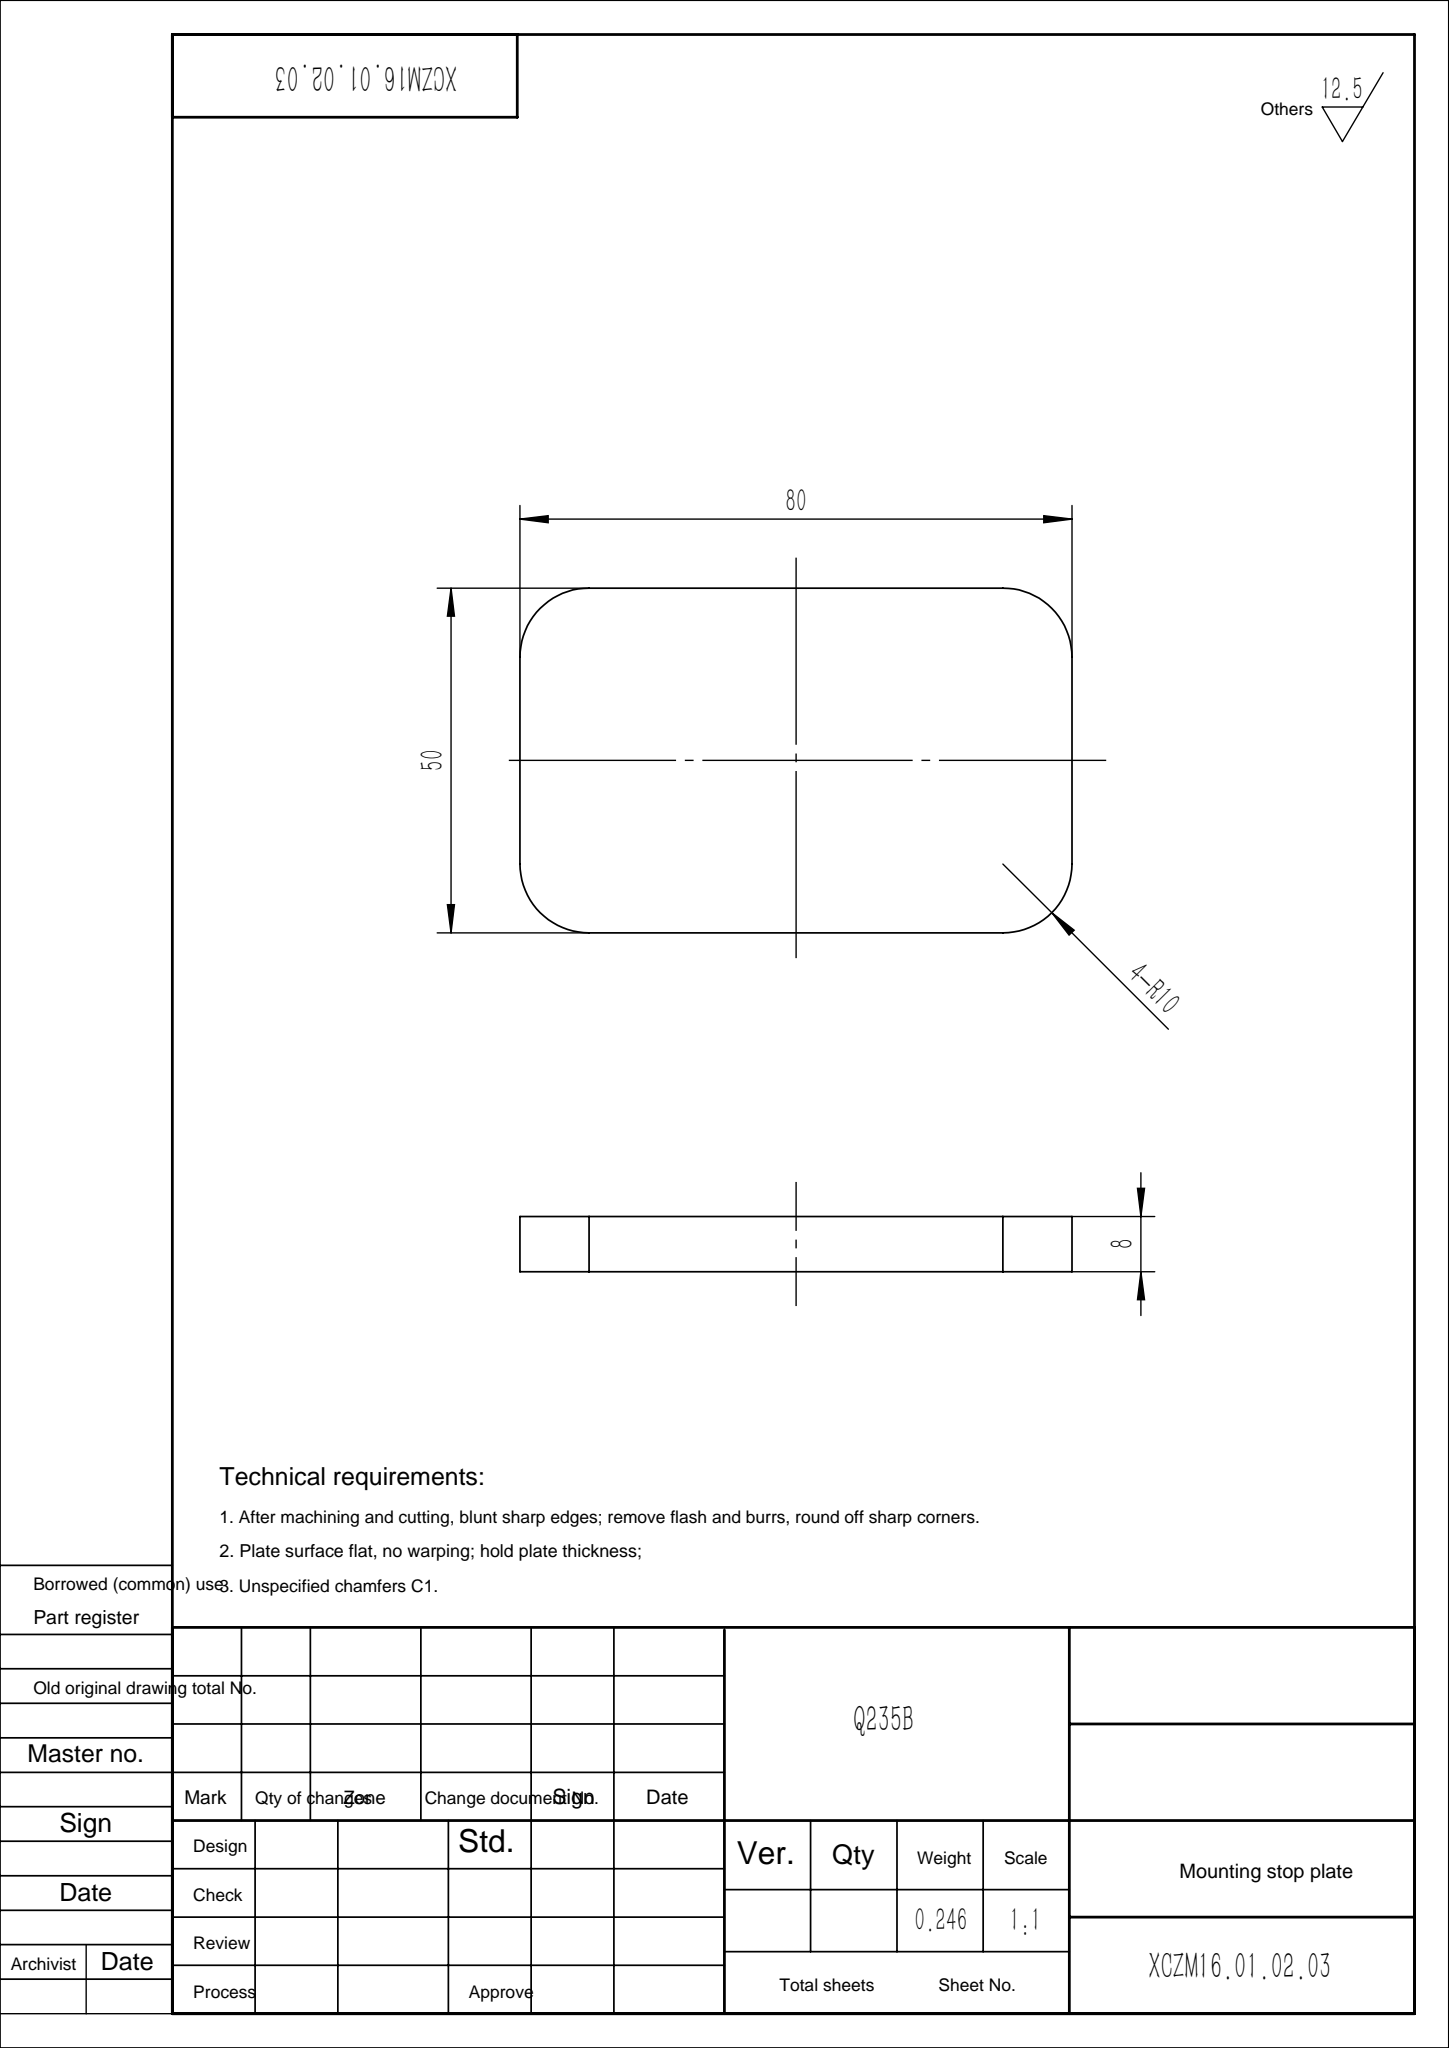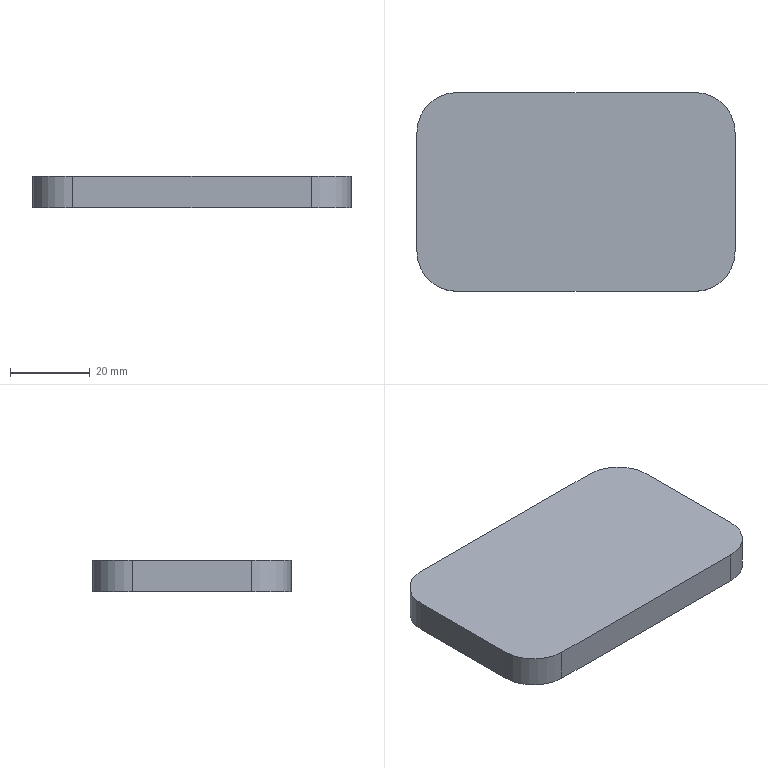Part | SolidWorks | features Extrusion 1 | 1 solid | 10 faces | box 80 x 50 x 8 mm | volume 31313 mm3 | plane 6 | cylinder 4 | commonest cylinder face diameters 20 x4
STEP:
#1=CARTESIAN_POINT('',(-40.,-15.,0.));
#2=VERTEX_POINT('',#1);
#3=CARTESIAN_POINT('',(-30.,-25.,0.));
#4=VERTEX_POINT('',#3);
#5=CARTESIAN_POINT('',(-30.,-15.,0.));
#6=DIRECTION('',(0.,0.,1.));
#7=DIRECTION('',(-1.,0.,0.));
#8=AXIS2_PLACEMENT_3D('',#5,#6,#7);
#9=CIRCLE('',#8,10.);
#10=EDGE_CURVE('',#2,#4,#9,.T.);
#11=ORIENTED_EDGE('',*,*,#10,.T.);
#12=CARTESIAN_POINT('',(-30.,-25.,8.));
#13=VERTEX_POINT('',#12);
#14=CARTESIAN_POINT('',(-30.,-25.,8.));
#15=DIRECTION('',(0.,0.,-1.));
#16=VECTOR('',#15,1000.);
#17=LINE('',#14,#16);
#18=EDGE_CURVE('',#13,#4,#17,.T.);
#19=ORIENTED_EDGE('',*,*,#18,.F.);
#20=CARTESIAN_POINT('',(-40.,-15.,8.));
#21=VERTEX_POINT('',#20);
#22=CARTESIAN_POINT('',(-30.,-15.,8.));
#23=DIRECTION('',(0.,0.,1.));
#24=DIRECTION('',(-1.,0.,0.));
#25=AXIS2_PLACEMENT_3D('',#22,#23,#24);
#26=CIRCLE('',#25,10.);
#27=EDGE_CURVE('',#21,#13,#26,.T.);
#28=ORIENTED_EDGE('',*,*,#27,.F.);
#29=CARTESIAN_POINT('',(-40.,-15.,8.));
#30=DIRECTION('',(0.,0.,-1.));
#31=VECTOR('',#30,1000.);
#32=LINE('',#29,#31);
#33=EDGE_CURVE('',#21,#2,#32,.T.);
#34=ORIENTED_EDGE('',*,*,#33,.T.);
#35=EDGE_LOOP('',(#11,#19,#28,#34));
#36=FACE_OUTER_BOUND('',#35,.T.);
#37=CARTESIAN_POINT('',(-30.,-15.,8.));
#38=DIRECTION('',(0.,0.,-1.));
#39=DIRECTION('',(-1.,0.,0.));
#40=AXIS2_PLACEMENT_3D('',#37,#38,#39);
#41=CYLINDRICAL_SURFACE('',#40,10.);
#42=ADVANCED_FACE('',(#36),#41,.T.);
#43=CARTESIAN_POINT('',(30.,-25.,0.));
#44=VERTEX_POINT('',#43);
#45=CARTESIAN_POINT('',(30.,-25.,0.));
#46=DIRECTION('',(1.,0.,0.));
#47=VECTOR('',#46,1000.);
#48=LINE('',#45,#47);
#49=EDGE_CURVE('',#4,#44,#48,.T.);
#50=ORIENTED_EDGE('',*,*,#49,.T.);
#51=CARTESIAN_POINT('',(30.,-25.,8.));
#52=VERTEX_POINT('',#51);
#53=CARTESIAN_POINT('',(30.,-25.,8.));
#54=DIRECTION('',(0.,0.,-1.));
#55=VECTOR('',#54,1000.);
#56=LINE('',#53,#55);
#57=EDGE_CURVE('',#52,#44,#56,.T.);
#58=ORIENTED_EDGE('',*,*,#57,.F.);
#59=CARTESIAN_POINT('',(30.,-25.,8.));
#60=DIRECTION('',(1.,0.,0.));
#61=VECTOR('',#60,1000.);
#62=LINE('',#59,#61);
#63=EDGE_CURVE('',#13,#52,#62,.T.);
#64=ORIENTED_EDGE('',*,*,#63,.F.);
#65=ORIENTED_EDGE('',*,*,#18,.T.);
#66=EDGE_LOOP('',(#50,#58,#64,#65));
#67=FACE_OUTER_BOUND('',#66,.T.);
#68=CARTESIAN_POINT('',(30.,-25.,8.));
#69=DIRECTION('',(0.,1.,0.));
#70=DIRECTION('',(-1.,0.,0.));
#71=AXIS2_PLACEMENT_3D('',#68,#69,#70);
#72=PLANE('',#71);
#73=ADVANCED_FACE('',(#67),#72,.F.);
#74=CARTESIAN_POINT('',(40.,-15.,0.));
#75=VERTEX_POINT('',#74);
#76=CARTESIAN_POINT('',(30.,-15.,0.));
#77=DIRECTION('',(0.,0.,1.));
#78=DIRECTION('',(1.,0.,0.));
#79=AXIS2_PLACEMENT_3D('',#76,#77,#78);
#80=CIRCLE('',#79,10.);
#81=EDGE_CURVE('',#44,#75,#80,.T.);
#82=ORIENTED_EDGE('',*,*,#81,.T.);
#83=CARTESIAN_POINT('',(40.,-15.,8.));
#84=VERTEX_POINT('',#83);
#85=CARTESIAN_POINT('',(40.,-15.,8.));
#86=DIRECTION('',(0.,0.,-1.));
#87=VECTOR('',#86,1000.);
#88=LINE('',#85,#87);
#89=EDGE_CURVE('',#84,#75,#88,.T.);
#90=ORIENTED_EDGE('',*,*,#89,.F.);
#91=CARTESIAN_POINT('',(30.,-15.,8.));
#92=DIRECTION('',(0.,0.,1.));
#93=DIRECTION('',(1.,0.,0.));
#94=AXIS2_PLACEMENT_3D('',#91,#92,#93);
#95=CIRCLE('',#94,10.);
#96=EDGE_CURVE('',#52,#84,#95,.T.);
#97=ORIENTED_EDGE('',*,*,#96,.F.);
#98=ORIENTED_EDGE('',*,*,#57,.T.);
#99=EDGE_LOOP('',(#82,#90,#97,#98));
#100=FACE_OUTER_BOUND('',#99,.T.);
#101=CARTESIAN_POINT('',(30.,-15.,8.));
#102=DIRECTION('',(0.,0.,-1.));
#103=DIRECTION('',(-1.,0.,0.));
#104=AXIS2_PLACEMENT_3D('',#101,#102,#103);
#105=CYLINDRICAL_SURFACE('',#104,10.);
#106=ADVANCED_FACE('',(#100),#105,.T.);
#107=CARTESIAN_POINT('',(40.,15.,0.));
#108=VERTEX_POINT('',#107);
#109=CARTESIAN_POINT('',(40.,-15.,0.));
#110=DIRECTION('',(0.,1.,0.));
#111=VECTOR('',#110,1000.);
#112=LINE('',#109,#111);
#113=EDGE_CURVE('',#75,#108,#112,.T.);
#114=ORIENTED_EDGE('',*,*,#113,.T.);
#115=CARTESIAN_POINT('',(40.,15.,8.));
#116=VERTEX_POINT('',#115);
#117=CARTESIAN_POINT('',(40.,15.,8.));
#118=DIRECTION('',(0.,0.,-1.));
#119=VECTOR('',#118,1000.);
#120=LINE('',#117,#119);
#121=EDGE_CURVE('',#116,#108,#120,.T.);
#122=ORIENTED_EDGE('',*,*,#121,.F.);
#123=CARTESIAN_POINT('',(40.,-15.,8.));
#124=DIRECTION('',(0.,1.,0.));
#125=VECTOR('',#124,1000.);
#126=LINE('',#123,#125);
#127=EDGE_CURVE('',#84,#116,#126,.T.);
#128=ORIENTED_EDGE('',*,*,#127,.F.);
#129=ORIENTED_EDGE('',*,*,#89,.T.);
#130=EDGE_LOOP('',(#114,#122,#128,#129));
#131=FACE_OUTER_BOUND('',#130,.T.);
#132=CARTESIAN_POINT('',(40.,-15.,8.));
#133=DIRECTION('',(-1.,0.,0.));
#134=DIRECTION('',(0.,0.,1.));
#135=AXIS2_PLACEMENT_3D('',#132,#133,#134);
#136=PLANE('',#135);
#137=ADVANCED_FACE('',(#131),#136,.F.);
#138=CARTESIAN_POINT('',(30.,25.,0.));
#139=VERTEX_POINT('',#138);
#140=CARTESIAN_POINT('',(30.,15.,0.));
#141=DIRECTION('',(0.,0.,1.));
#142=DIRECTION('',(1.,0.,0.));
#143=AXIS2_PLACEMENT_3D('',#140,#141,#142);
#144=CIRCLE('',#143,10.);
#145=EDGE_CURVE('',#108,#139,#144,.T.);
#146=ORIENTED_EDGE('',*,*,#145,.T.);
#147=CARTESIAN_POINT('',(30.,25.,8.));
#148=VERTEX_POINT('',#147);
#149=CARTESIAN_POINT('',(30.,25.,8.));
#150=DIRECTION('',(0.,0.,-1.));
#151=VECTOR('',#150,1000.);
#152=LINE('',#149,#151);
#153=EDGE_CURVE('',#148,#139,#152,.T.);
#154=ORIENTED_EDGE('',*,*,#153,.F.);
#155=CARTESIAN_POINT('',(30.,15.,8.));
#156=DIRECTION('',(0.,0.,1.));
#157=DIRECTION('',(1.,0.,0.));
#158=AXIS2_PLACEMENT_3D('',#155,#156,#157);
#159=CIRCLE('',#158,10.);
#160=EDGE_CURVE('',#116,#148,#159,.T.);
#161=ORIENTED_EDGE('',*,*,#160,.F.);
#162=ORIENTED_EDGE('',*,*,#121,.T.);
#163=EDGE_LOOP('',(#146,#154,#161,#162));
#164=FACE_OUTER_BOUND('',#163,.T.);
#165=CARTESIAN_POINT('',(30.,15.,8.));
#166=DIRECTION('',(0.,0.,-1.));
#167=DIRECTION('',(-1.,0.,0.));
#168=AXIS2_PLACEMENT_3D('',#165,#166,#167);
#169=CYLINDRICAL_SURFACE('',#168,10.);
#170=ADVANCED_FACE('',(#164),#169,.T.);
#171=CARTESIAN_POINT('',(-30.,25.,0.));
#172=VERTEX_POINT('',#171);
#173=CARTESIAN_POINT('',(30.,25.,0.));
#174=DIRECTION('',(-1.,0.,0.));
#175=VECTOR('',#174,1000.);
#176=LINE('',#173,#175);
#177=EDGE_CURVE('',#139,#172,#176,.T.);
#178=ORIENTED_EDGE('',*,*,#177,.T.);
#179=CARTESIAN_POINT('',(-30.,25.,8.));
#180=VERTEX_POINT('',#179);
#181=CARTESIAN_POINT('',(-30.,25.,8.));
#182=DIRECTION('',(0.,0.,-1.));
#183=VECTOR('',#182,1000.);
#184=LINE('',#181,#183);
#185=EDGE_CURVE('',#180,#172,#184,.T.);
#186=ORIENTED_EDGE('',*,*,#185,.F.);
#187=CARTESIAN_POINT('',(30.,25.,8.));
#188=DIRECTION('',(-1.,0.,0.));
#189=VECTOR('',#188,1000.);
#190=LINE('',#187,#189);
#191=EDGE_CURVE('',#148,#180,#190,.T.);
#192=ORIENTED_EDGE('',*,*,#191,.F.);
#193=ORIENTED_EDGE('',*,*,#153,.T.);
#194=EDGE_LOOP('',(#178,#186,#192,#193));
#195=FACE_OUTER_BOUND('',#194,.T.);
#196=CARTESIAN_POINT('',(30.,25.,8.));
#197=DIRECTION('',(0.,-1.,0.));
#198=DIRECTION('',(1.,0.,0.));
#199=AXIS2_PLACEMENT_3D('',#196,#197,#198);
#200=PLANE('',#199);
#201=ADVANCED_FACE('',(#195),#200,.F.);
#202=CARTESIAN_POINT('',(-40.,15.,0.));
#203=VERTEX_POINT('',#202);
#204=CARTESIAN_POINT('',(-30.,15.,0.));
#205=DIRECTION('',(0.,0.,1.));
#206=DIRECTION('',(1.,0.,0.));
#207=AXIS2_PLACEMENT_3D('',#204,#205,#206);
#208=CIRCLE('',#207,10.);
#209=EDGE_CURVE('',#172,#203,#208,.T.);
#210=ORIENTED_EDGE('',*,*,#209,.T.);
#211=CARTESIAN_POINT('',(-40.,15.,8.));
#212=VERTEX_POINT('',#211);
#213=CARTESIAN_POINT('',(-40.,15.,8.));
#214=DIRECTION('',(0.,0.,-1.));
#215=VECTOR('',#214,1000.);
#216=LINE('',#213,#215);
#217=EDGE_CURVE('',#212,#203,#216,.T.);
#218=ORIENTED_EDGE('',*,*,#217,.F.);
#219=CARTESIAN_POINT('',(-30.,15.,8.));
#220=DIRECTION('',(0.,0.,1.));
#221=DIRECTION('',(1.,0.,0.));
#222=AXIS2_PLACEMENT_3D('',#219,#220,#221);
#223=CIRCLE('',#222,10.);
#224=EDGE_CURVE('',#180,#212,#223,.T.);
#225=ORIENTED_EDGE('',*,*,#224,.F.);
#226=ORIENTED_EDGE('',*,*,#185,.T.);
#227=EDGE_LOOP('',(#210,#218,#225,#226));
#228=FACE_OUTER_BOUND('',#227,.T.);
#229=CARTESIAN_POINT('',(-30.,15.,8.));
#230=DIRECTION('',(0.,0.,-1.));
#231=DIRECTION('',(-1.,0.,0.));
#232=AXIS2_PLACEMENT_3D('',#229,#230,#231);
#233=CYLINDRICAL_SURFACE('',#232,10.);
#234=ADVANCED_FACE('',(#228),#233,.T.);
#235=CARTESIAN_POINT('',(-40.,-15.,0.));
#236=DIRECTION('',(0.,-1.,0.));
#237=VECTOR('',#236,1000.);
#238=LINE('',#235,#237);
#239=EDGE_CURVE('',#203,#2,#238,.T.);
#240=ORIENTED_EDGE('',*,*,#239,.T.);
#241=ORIENTED_EDGE('',*,*,#33,.F.);
#242=CARTESIAN_POINT('',(-40.,-15.,8.));
#243=DIRECTION('',(0.,-1.,0.));
#244=VECTOR('',#243,1000.);
#245=LINE('',#242,#244);
#246=EDGE_CURVE('',#212,#21,#245,.T.);
#247=ORIENTED_EDGE('',*,*,#246,.F.);
#248=ORIENTED_EDGE('',*,*,#217,.T.);
#249=EDGE_LOOP('',(#240,#241,#247,#248));
#250=FACE_OUTER_BOUND('',#249,.T.);
#251=CARTESIAN_POINT('',(-40.,-15.,8.));
#252=DIRECTION('',(1.,0.,0.));
#253=DIRECTION('',(0.,1.,0.));
#254=AXIS2_PLACEMENT_3D('',#251,#252,#253);
#255=PLANE('',#254);
#256=ADVANCED_FACE('',(#250),#255,.F.);
#257=ORIENTED_EDGE('',*,*,#27,.T.);
#258=ORIENTED_EDGE('',*,*,#63,.T.);
#259=ORIENTED_EDGE('',*,*,#96,.T.);
#260=ORIENTED_EDGE('',*,*,#127,.T.);
#261=ORIENTED_EDGE('',*,*,#160,.T.);
#262=ORIENTED_EDGE('',*,*,#191,.T.);
#263=ORIENTED_EDGE('',*,*,#224,.T.);
#264=ORIENTED_EDGE('',*,*,#246,.T.);
#265=EDGE_LOOP('',(#257,#258,#259,#260,#261,#262,#263,#264));
#266=FACE_OUTER_BOUND('',#265,.T.);
#267=CARTESIAN_POINT('',(-30.,-15.,8.));
#268=DIRECTION('',(0.,0.,-1.));
#269=DIRECTION('',(-1.,0.,0.));
#270=AXIS2_PLACEMENT_3D('',#267,#268,#269);
#271=PLANE('',#270);
#272=ADVANCED_FACE('',(#266),#271,.F.);
#273=ORIENTED_EDGE('',*,*,#10,.F.);
#274=ORIENTED_EDGE('',*,*,#239,.F.);
#275=ORIENTED_EDGE('',*,*,#209,.F.);
#276=ORIENTED_EDGE('',*,*,#177,.F.);
#277=ORIENTED_EDGE('',*,*,#145,.F.);
#278=ORIENTED_EDGE('',*,*,#113,.F.);
#279=ORIENTED_EDGE('',*,*,#81,.F.);
#280=ORIENTED_EDGE('',*,*,#49,.F.);
#281=EDGE_LOOP('',(#273,#274,#275,#276,#277,#278,#279,#280));
#282=FACE_OUTER_BOUND('',#281,.T.);
#283=CARTESIAN_POINT('',(-30.,-15.,0.));
#284=DIRECTION('',(0.,0.,-1.));
#285=DIRECTION('',(-1.,0.,0.));
#286=AXIS2_PLACEMENT_3D('',#283,#284,#285);
#287=PLANE('',#286);
#288=ADVANCED_FACE('',(#282),#287,.T.);
#289=CLOSED_SHELL('',(#42,#73,#106,#137,#170,#201,#234,#256,#272,#288));
#290=MANIFOLD_SOLID_BREP('',#289);
#291=CARTESIAN_POINT('',(0.,0.,0.));
#292=DIRECTION('',(0.,0.,1.));
#293=DIRECTION('',(1.,0.,0.));
#294=AXIS2_PLACEMENT_3D('',#291,#292,#293);
#295=(LENGTH_UNIT()NAMED_UNIT(*)SI_UNIT(.MILLI.,.METRE.));
#296=UNCERTAINTY_MEASURE_WITH_UNIT(LENGTH_MEASURE(0.00001),#295,'','');
#297=(NAMED_UNIT(*)PLANE_ANGLE_UNIT()SI_UNIT($,.RADIAN.));
#298=(NAMED_UNIT(*)SI_UNIT($,.STERADIAN.)SOLID_ANGLE_UNIT());
#299=(GEOMETRIC_REPRESENTATION_CONTEXT(3)GLOBAL_UNCERTAINTY_ASSIGNED_CONTEXT((#296))GLOBAL_UNIT_ASSIGNED_CONTEXT((#295,#297,#298))REPRESENTATION_CONTEXT('',''));
#300=ADVANCED_BREP_SHAPE_REPRESENTATION('',(#290,#294),#299);